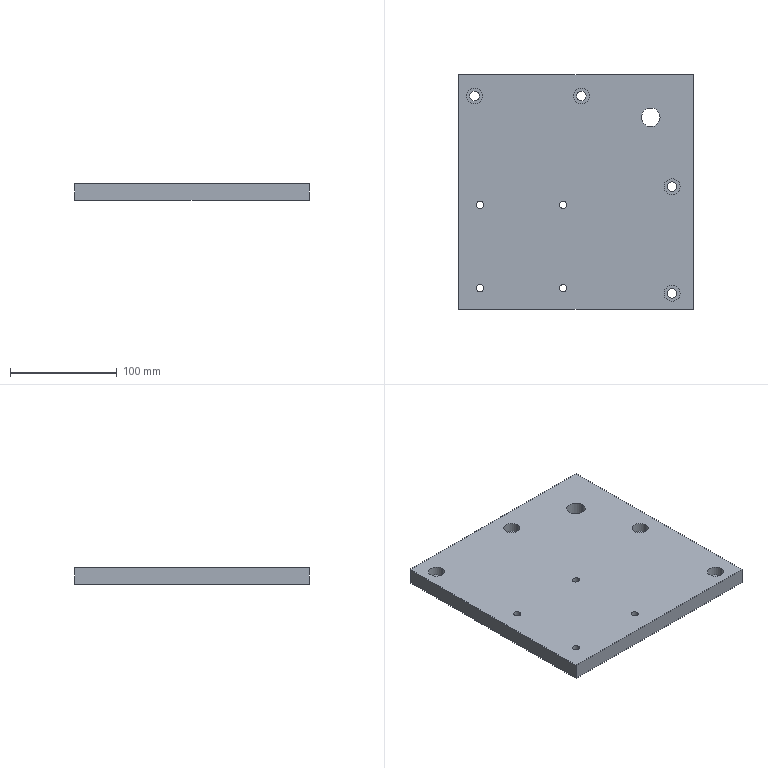Part | SolidWorks | features BaseBody 1 | 1 solid | 36 faces | box 220 x 220 x 15 mm | volume 712325 mm3 | cylinder 26 | plane 10 | commonest cylinder face diameters 6.8 x8 9 x8 15 x8 17.5 x2
STEP:
#1=CARTESIAN_POINT('',(82.5,-95.,6.));
#2=VERTEX_POINT('',#1);
#3=CARTESIAN_POINT('',(97.5,-95.,6.));
#4=VERTEX_POINT('',#3);
#5=CARTESIAN_POINT('',(90.,-95.,6.));
#6=DIRECTION('',(0.,0.,1.));
#7=DIRECTION('',(1.,0.,0.));
#8=AXIS2_PLACEMENT_3D('',#5,#6,#7);
#9=CIRCLE('',#8,7.5);
#10=EDGE_CURVE('',#2,#4,#9,.T.);
#11=ORIENTED_EDGE('',*,*,#10,.F.);
#12=CARTESIAN_POINT('',(82.5,-95.,15.));
#13=VERTEX_POINT('',#12);
#14=CARTESIAN_POINT('',(82.5,-95.,15.));
#15=DIRECTION('',(0.,0.,1.));
#16=VECTOR('',#15,1000.);
#17=LINE('',#14,#16);
#18=EDGE_CURVE('',#2,#13,#17,.T.);
#19=ORIENTED_EDGE('',*,*,#18,.T.);
#20=CARTESIAN_POINT('',(97.5,-95.,15.));
#21=VERTEX_POINT('',#20);
#22=CARTESIAN_POINT('',(90.,-95.,15.));
#23=DIRECTION('',(0.,0.,1.));
#24=DIRECTION('',(1.,0.,0.));
#25=AXIS2_PLACEMENT_3D('',#22,#23,#24);
#26=CIRCLE('',#25,7.5);
#27=EDGE_CURVE('',#13,#21,#26,.T.);
#28=ORIENTED_EDGE('',*,*,#27,.T.);
#29=CARTESIAN_POINT('',(97.5,-95.,15.));
#30=DIRECTION('',(0.,0.,1.));
#31=VECTOR('',#30,1000.);
#32=LINE('',#29,#31);
#33=EDGE_CURVE('',#4,#21,#32,.T.);
#34=ORIENTED_EDGE('',*,*,#33,.F.);
#35=EDGE_LOOP('',(#11,#19,#28,#34));
#36=FACE_OUTER_BOUND('',#35,.T.);
#37=CARTESIAN_POINT('',(90.,-95.,15.));
#38=DIRECTION('',(0.,0.,1.));
#39=DIRECTION('',(1.,0.,0.));
#40=AXIS2_PLACEMENT_3D('',#37,#38,#39);
#41=CYLINDRICAL_SURFACE('',#40,7.5);
#42=ADVANCED_FACE('',(#36),#41,.F.);
#43=CARTESIAN_POINT('',(85.5,-95.,0.));
#44=VERTEX_POINT('',#43);
#45=CARTESIAN_POINT('',(94.5,-95.,0.));
#46=VERTEX_POINT('',#45);
#47=CARTESIAN_POINT('',(90.,-95.,0.));
#48=DIRECTION('',(0.,0.,1.));
#49=DIRECTION('',(1.,0.,0.));
#50=AXIS2_PLACEMENT_3D('',#47,#48,#49);
#51=CIRCLE('',#50,4.5);
#52=EDGE_CURVE('',#44,#46,#51,.T.);
#53=ORIENTED_EDGE('',*,*,#52,.F.);
#54=CARTESIAN_POINT('',(85.5,-95.,6.));
#55=VERTEX_POINT('',#54);
#56=CARTESIAN_POINT('',(85.5,-95.,15.));
#57=DIRECTION('',(0.,0.,1.));
#58=VECTOR('',#57,1000.);
#59=LINE('',#56,#58);
#60=EDGE_CURVE('',#44,#55,#59,.T.);
#61=ORIENTED_EDGE('',*,*,#60,.T.);
#62=CARTESIAN_POINT('',(94.5,-95.,6.));
#63=VERTEX_POINT('',#62);
#64=CARTESIAN_POINT('',(90.,-95.,6.));
#65=DIRECTION('',(0.,0.,1.));
#66=DIRECTION('',(1.,0.,0.));
#67=AXIS2_PLACEMENT_3D('',#64,#65,#66);
#68=CIRCLE('',#67,4.5);
#69=EDGE_CURVE('',#55,#63,#68,.T.);
#70=ORIENTED_EDGE('',*,*,#69,.T.);
#71=CARTESIAN_POINT('',(94.5,-95.,15.));
#72=DIRECTION('',(0.,0.,1.));
#73=VECTOR('',#72,1000.);
#74=LINE('',#71,#73);
#75=EDGE_CURVE('',#46,#63,#74,.T.);
#76=ORIENTED_EDGE('',*,*,#75,.F.);
#77=EDGE_LOOP('',(#53,#61,#70,#76));
#78=FACE_OUTER_BOUND('',#77,.T.);
#79=CARTESIAN_POINT('',(90.,-95.,15.));
#80=DIRECTION('',(0.,0.,1.));
#81=DIRECTION('',(1.,0.,0.));
#82=AXIS2_PLACEMENT_3D('',#79,#80,#81);
#83=CYLINDRICAL_SURFACE('',#82,4.5);
#84=ADVANCED_FACE('',(#78),#83,.F.);
#85=CARTESIAN_POINT('',(82.5,5.,6.));
#86=VERTEX_POINT('',#85);
#87=CARTESIAN_POINT('',(97.5,5.,6.));
#88=VERTEX_POINT('',#87);
#89=CARTESIAN_POINT('',(90.,5.,6.));
#90=DIRECTION('',(0.,0.,1.));
#91=DIRECTION('',(1.,0.,0.));
#92=AXIS2_PLACEMENT_3D('',#89,#90,#91);
#93=CIRCLE('',#92,7.5);
#94=EDGE_CURVE('',#86,#88,#93,.T.);
#95=ORIENTED_EDGE('',*,*,#94,.F.);
#96=CARTESIAN_POINT('',(82.5,5.,15.));
#97=VERTEX_POINT('',#96);
#98=CARTESIAN_POINT('',(82.5,5.,15.));
#99=DIRECTION('',(0.,0.,1.));
#100=VECTOR('',#99,1000.);
#101=LINE('',#98,#100);
#102=EDGE_CURVE('',#86,#97,#101,.T.);
#103=ORIENTED_EDGE('',*,*,#102,.T.);
#104=CARTESIAN_POINT('',(97.5,5.,15.));
#105=VERTEX_POINT('',#104);
#106=CARTESIAN_POINT('',(90.,5.,15.));
#107=DIRECTION('',(0.,0.,1.));
#108=DIRECTION('',(1.,0.,0.));
#109=AXIS2_PLACEMENT_3D('',#106,#107,#108);
#110=CIRCLE('',#109,7.5);
#111=EDGE_CURVE('',#97,#105,#110,.T.);
#112=ORIENTED_EDGE('',*,*,#111,.T.);
#113=CARTESIAN_POINT('',(97.5,5.,15.));
#114=DIRECTION('',(0.,0.,1.));
#115=VECTOR('',#114,1000.);
#116=LINE('',#113,#115);
#117=EDGE_CURVE('',#88,#105,#116,.T.);
#118=ORIENTED_EDGE('',*,*,#117,.F.);
#119=EDGE_LOOP('',(#95,#103,#112,#118));
#120=FACE_OUTER_BOUND('',#119,.T.);
#121=CARTESIAN_POINT('',(90.,5.,15.));
#122=DIRECTION('',(0.,0.,1.));
#123=DIRECTION('',(1.,0.,0.));
#124=AXIS2_PLACEMENT_3D('',#121,#122,#123);
#125=CYLINDRICAL_SURFACE('',#124,7.5);
#126=ADVANCED_FACE('',(#120),#125,.F.);
#127=CARTESIAN_POINT('',(85.5,5.,0.));
#128=VERTEX_POINT('',#127);
#129=CARTESIAN_POINT('',(94.5,5.,0.));
#130=VERTEX_POINT('',#129);
#131=CARTESIAN_POINT('',(90.,5.,0.));
#132=DIRECTION('',(0.,0.,1.));
#133=DIRECTION('',(1.,0.,0.));
#134=AXIS2_PLACEMENT_3D('',#131,#132,#133);
#135=CIRCLE('',#134,4.5);
#136=EDGE_CURVE('',#128,#130,#135,.T.);
#137=ORIENTED_EDGE('',*,*,#136,.F.);
#138=CARTESIAN_POINT('',(85.5,5.,6.));
#139=VERTEX_POINT('',#138);
#140=CARTESIAN_POINT('',(85.5,5.,15.));
#141=DIRECTION('',(0.,0.,1.));
#142=VECTOR('',#141,1000.);
#143=LINE('',#140,#142);
#144=EDGE_CURVE('',#128,#139,#143,.T.);
#145=ORIENTED_EDGE('',*,*,#144,.T.);
#146=CARTESIAN_POINT('',(94.5,5.,6.));
#147=VERTEX_POINT('',#146);
#148=CARTESIAN_POINT('',(90.,5.,6.));
#149=DIRECTION('',(0.,0.,1.));
#150=DIRECTION('',(1.,0.,0.));
#151=AXIS2_PLACEMENT_3D('',#148,#149,#150);
#152=CIRCLE('',#151,4.5);
#153=EDGE_CURVE('',#139,#147,#152,.T.);
#154=ORIENTED_EDGE('',*,*,#153,.T.);
#155=CARTESIAN_POINT('',(94.5,5.,15.));
#156=DIRECTION('',(0.,0.,1.));
#157=VECTOR('',#156,1000.);
#158=LINE('',#155,#157);
#159=EDGE_CURVE('',#130,#147,#158,.T.);
#160=ORIENTED_EDGE('',*,*,#159,.F.);
#161=EDGE_LOOP('',(#137,#145,#154,#160));
#162=FACE_OUTER_BOUND('',#161,.T.);
#163=CARTESIAN_POINT('',(90.,5.,15.));
#164=DIRECTION('',(0.,0.,1.));
#165=DIRECTION('',(1.,0.,0.));
#166=AXIS2_PLACEMENT_3D('',#163,#164,#165);
#167=CYLINDRICAL_SURFACE('',#166,4.5);
#168=ADVANCED_FACE('',(#162),#167,.F.);
#169=CARTESIAN_POINT('',(-102.5,90.,6.));
#170=VERTEX_POINT('',#169);
#171=CARTESIAN_POINT('',(-87.5,90.,6.));
#172=VERTEX_POINT('',#171);
#173=CARTESIAN_POINT('',(-95.,90.,6.));
#174=DIRECTION('',(0.,0.,1.));
#175=DIRECTION('',(1.,0.,0.));
#176=AXIS2_PLACEMENT_3D('',#173,#174,#175);
#177=CIRCLE('',#176,7.5);
#178=EDGE_CURVE('',#170,#172,#177,.T.);
#179=ORIENTED_EDGE('',*,*,#178,.F.);
#180=CARTESIAN_POINT('',(-102.5,90.,15.));
#181=VERTEX_POINT('',#180);
#182=CARTESIAN_POINT('',(-102.5,90.,15.));
#183=DIRECTION('',(0.,0.,1.));
#184=VECTOR('',#183,1000.);
#185=LINE('',#182,#184);
#186=EDGE_CURVE('',#170,#181,#185,.T.);
#187=ORIENTED_EDGE('',*,*,#186,.T.);
#188=CARTESIAN_POINT('',(-87.5,90.,15.));
#189=VERTEX_POINT('',#188);
#190=CARTESIAN_POINT('',(-95.,90.,15.));
#191=DIRECTION('',(0.,0.,1.));
#192=DIRECTION('',(1.,0.,0.));
#193=AXIS2_PLACEMENT_3D('',#190,#191,#192);
#194=CIRCLE('',#193,7.5);
#195=EDGE_CURVE('',#181,#189,#194,.T.);
#196=ORIENTED_EDGE('',*,*,#195,.T.);
#197=CARTESIAN_POINT('',(-87.5,90.,15.));
#198=DIRECTION('',(0.,0.,1.));
#199=VECTOR('',#198,1000.);
#200=LINE('',#197,#199);
#201=EDGE_CURVE('',#172,#189,#200,.T.);
#202=ORIENTED_EDGE('',*,*,#201,.F.);
#203=EDGE_LOOP('',(#179,#187,#196,#202));
#204=FACE_OUTER_BOUND('',#203,.T.);
#205=CARTESIAN_POINT('',(-95.,90.,15.));
#206=DIRECTION('',(0.,0.,1.));
#207=DIRECTION('',(1.,0.,0.));
#208=AXIS2_PLACEMENT_3D('',#205,#206,#207);
#209=CYLINDRICAL_SURFACE('',#208,7.5);
#210=ADVANCED_FACE('',(#204),#209,.F.);
#211=CARTESIAN_POINT('',(-99.5,90.,0.));
#212=VERTEX_POINT('',#211);
#213=CARTESIAN_POINT('',(-90.5,90.,0.));
#214=VERTEX_POINT('',#213);
#215=CARTESIAN_POINT('',(-95.,90.,0.));
#216=DIRECTION('',(0.,0.,1.));
#217=DIRECTION('',(1.,0.,0.));
#218=AXIS2_PLACEMENT_3D('',#215,#216,#217);
#219=CIRCLE('',#218,4.5);
#220=EDGE_CURVE('',#212,#214,#219,.T.);
#221=ORIENTED_EDGE('',*,*,#220,.F.);
#222=CARTESIAN_POINT('',(-99.5,90.,6.));
#223=VERTEX_POINT('',#222);
#224=CARTESIAN_POINT('',(-99.5,90.,15.));
#225=DIRECTION('',(0.,0.,1.));
#226=VECTOR('',#225,1000.);
#227=LINE('',#224,#226);
#228=EDGE_CURVE('',#212,#223,#227,.T.);
#229=ORIENTED_EDGE('',*,*,#228,.T.);
#230=CARTESIAN_POINT('',(-90.5,90.,6.));
#231=VERTEX_POINT('',#230);
#232=CARTESIAN_POINT('',(-95.,90.,6.));
#233=DIRECTION('',(0.,0.,1.));
#234=DIRECTION('',(1.,0.,0.));
#235=AXIS2_PLACEMENT_3D('',#232,#233,#234);
#236=CIRCLE('',#235,4.5);
#237=EDGE_CURVE('',#223,#231,#236,.T.);
#238=ORIENTED_EDGE('',*,*,#237,.T.);
#239=CARTESIAN_POINT('',(-90.5,90.,15.));
#240=DIRECTION('',(0.,0.,1.));
#241=VECTOR('',#240,1000.);
#242=LINE('',#239,#241);
#243=EDGE_CURVE('',#214,#231,#242,.T.);
#244=ORIENTED_EDGE('',*,*,#243,.F.);
#245=EDGE_LOOP('',(#221,#229,#238,#244));
#246=FACE_OUTER_BOUND('',#245,.T.);
#247=CARTESIAN_POINT('',(-95.,90.,15.));
#248=DIRECTION('',(0.,0.,1.));
#249=DIRECTION('',(1.,0.,0.));
#250=AXIS2_PLACEMENT_3D('',#247,#248,#249);
#251=CYLINDRICAL_SURFACE('',#250,4.5);
#252=ADVANCED_FACE('',(#246),#251,.F.);
#253=CARTESIAN_POINT('',(-2.5,90.,6.));
#254=VERTEX_POINT('',#253);
#255=CARTESIAN_POINT('',(12.5,90.,6.));
#256=VERTEX_POINT('',#255);
#257=CARTESIAN_POINT('',(5.,90.,6.));
#258=DIRECTION('',(0.,0.,1.));
#259=DIRECTION('',(1.,0.,0.));
#260=AXIS2_PLACEMENT_3D('',#257,#258,#259);
#261=CIRCLE('',#260,7.5);
#262=EDGE_CURVE('',#254,#256,#261,.T.);
#263=ORIENTED_EDGE('',*,*,#262,.F.);
#264=CARTESIAN_POINT('',(-2.5,90.,15.));
#265=VERTEX_POINT('',#264);
#266=CARTESIAN_POINT('',(-2.5,90.,15.));
#267=DIRECTION('',(0.,0.,1.));
#268=VECTOR('',#267,1000.);
#269=LINE('',#266,#268);
#270=EDGE_CURVE('',#254,#265,#269,.T.);
#271=ORIENTED_EDGE('',*,*,#270,.T.);
#272=CARTESIAN_POINT('',(12.5,90.,15.));
#273=VERTEX_POINT('',#272);
#274=CARTESIAN_POINT('',(5.,90.,15.));
#275=DIRECTION('',(0.,0.,1.));
#276=DIRECTION('',(1.,0.,0.));
#277=AXIS2_PLACEMENT_3D('',#274,#275,#276);
#278=CIRCLE('',#277,7.5);
#279=EDGE_CURVE('',#265,#273,#278,.T.);
#280=ORIENTED_EDGE('',*,*,#279,.T.);
#281=CARTESIAN_POINT('',(12.5,90.,15.));
#282=DIRECTION('',(0.,0.,1.));
#283=VECTOR('',#282,1000.);
#284=LINE('',#281,#283);
#285=EDGE_CURVE('',#256,#273,#284,.T.);
#286=ORIENTED_EDGE('',*,*,#285,.F.);
#287=EDGE_LOOP('',(#263,#271,#280,#286));
#288=FACE_OUTER_BOUND('',#287,.T.);
#289=CARTESIAN_POINT('',(5.,90.,15.));
#290=DIRECTION('',(0.,0.,1.));
#291=DIRECTION('',(1.,0.,0.));
#292=AXIS2_PLACEMENT_3D('',#289,#290,#291);
#293=CYLINDRICAL_SURFACE('',#292,7.5);
#294=ADVANCED_FACE('',(#288),#293,.F.);
#295=CARTESIAN_POINT('',(0.5,90.,0.));
#296=VERTEX_POINT('',#295);
#297=CARTESIAN_POINT('',(9.5,90.,0.));
#298=VERTEX_POINT('',#297);
#299=CARTESIAN_POINT('',(5.,90.,0.));
#300=DIRECTION('',(0.,0.,1.));
#301=DIRECTION('',(1.,0.,0.));
#302=AXIS2_PLACEMENT_3D('',#299,#300,#301);
#303=CIRCLE('',#302,4.5);
#304=EDGE_CURVE('',#296,#298,#303,.T.);
#305=ORIENTED_EDGE('',*,*,#304,.F.);
#306=CARTESIAN_POINT('',(0.5,90.,6.));
#307=VERTEX_POINT('',#306);
#308=CARTESIAN_POINT('',(0.5,90.,15.));
#309=DIRECTION('',(0.,0.,1.));
#310=VECTOR('',#309,1000.);
#311=LINE('',#308,#310);
#312=EDGE_CURVE('',#296,#307,#311,.T.);
#313=ORIENTED_EDGE('',*,*,#312,.T.);
#314=CARTESIAN_POINT('',(9.5,90.,6.));
#315=VERTEX_POINT('',#314);
#316=CARTESIAN_POINT('',(5.,90.,6.));
#317=DIRECTION('',(0.,0.,1.));
#318=DIRECTION('',(1.,0.,0.));
#319=AXIS2_PLACEMENT_3D('',#316,#317,#318);
#320=CIRCLE('',#319,4.5);
#321=EDGE_CURVE('',#307,#315,#320,.T.);
#322=ORIENTED_EDGE('',*,*,#321,.T.);
#323=CARTESIAN_POINT('',(9.5,90.,15.));
#324=DIRECTION('',(0.,0.,1.));
#325=VECTOR('',#324,1000.);
#326=LINE('',#323,#325);
#327=EDGE_CURVE('',#298,#315,#326,.T.);
#328=ORIENTED_EDGE('',*,*,#327,.F.);
#329=EDGE_LOOP('',(#305,#313,#322,#328));
#330=FACE_OUTER_BOUND('',#329,.T.);
#331=CARTESIAN_POINT('',(5.,90.,15.));
#332=DIRECTION('',(0.,0.,1.));
#333=DIRECTION('',(1.,0.,0.));
#334=AXIS2_PLACEMENT_3D('',#331,#332,#333);
#335=CYLINDRICAL_SURFACE('',#334,4.5);
#336=ADVANCED_FACE('',(#330),#335,.F.);
#337=CARTESIAN_POINT('',(61.25,70.,0.));
#338=VERTEX_POINT('',#337);
#339=CARTESIAN_POINT('',(78.75,70.,0.));
#340=VERTEX_POINT('',#339);
#341=CARTESIAN_POINT('',(70.,70.,0.));
#342=DIRECTION('',(0.,0.,1.));
#343=DIRECTION('',(1.,0.,0.));
#344=AXIS2_PLACEMENT_3D('',#341,#342,#343);
#345=CIRCLE('',#344,8.75);
#346=EDGE_CURVE('',#338,#340,#345,.T.);
#347=ORIENTED_EDGE('',*,*,#346,.F.);
#348=CARTESIAN_POINT('',(61.25,70.,15.));
#349=VERTEX_POINT('',#348);
#350=CARTESIAN_POINT('',(61.25,70.,15.));
#351=DIRECTION('',(0.,0.,1.));
#352=VECTOR('',#351,1000.);
#353=LINE('',#350,#352);
#354=EDGE_CURVE('',#338,#349,#353,.T.);
#355=ORIENTED_EDGE('',*,*,#354,.T.);
#356=CARTESIAN_POINT('',(78.75,70.,15.));
#357=VERTEX_POINT('',#356);
#358=CARTESIAN_POINT('',(70.,70.,15.));
#359=DIRECTION('',(0.,0.,1.));
#360=DIRECTION('',(1.,0.,0.));
#361=AXIS2_PLACEMENT_3D('',#358,#359,#360);
#362=CIRCLE('',#361,8.75);
#363=EDGE_CURVE('',#349,#357,#362,.T.);
#364=ORIENTED_EDGE('',*,*,#363,.T.);
#365=CARTESIAN_POINT('',(78.75,70.,15.));
#366=DIRECTION('',(0.,0.,1.));
#367=VECTOR('',#366,1000.);
#368=LINE('',#365,#367);
#369=EDGE_CURVE('',#340,#357,#368,.T.);
#370=ORIENTED_EDGE('',*,*,#369,.F.);
#371=EDGE_LOOP('',(#347,#355,#364,#370));
#372=FACE_OUTER_BOUND('',#371,.T.);
#373=CARTESIAN_POINT('',(70.,70.,15.));
#374=DIRECTION('',(0.,0.,1.));
#375=DIRECTION('',(1.,0.,0.));
#376=AXIS2_PLACEMENT_3D('',#373,#374,#375);
#377=CYLINDRICAL_SURFACE('',#376,8.75);
#378=ADVANCED_FACE('',(#372),#377,.F.);
#379=CARTESIAN_POINT('',(-93.4,-90.,0.));
#380=VERTEX_POINT('',#379);
#381=CARTESIAN_POINT('',(-86.6,-90.,0.));
#382=VERTEX_POINT('',#381);
#383=CARTESIAN_POINT('',(-90.,-90.,0.));
#384=DIRECTION('',(0.,0.,1.));
#385=DIRECTION('',(1.,0.,0.));
#386=AXIS2_PLACEMENT_3D('',#383,#384,#385);
#387=CIRCLE('',#386,3.4);
#388=EDGE_CURVE('',#380,#382,#387,.T.);
#389=ORIENTED_EDGE('',*,*,#388,.F.);
#390=CARTESIAN_POINT('',(-93.4,-90.,15.));
#391=VERTEX_POINT('',#390);
#392=CARTESIAN_POINT('',(-93.4,-90.,15.));
#393=DIRECTION('',(0.,0.,1.));
#394=VECTOR('',#393,1000.);
#395=LINE('',#392,#394);
#396=EDGE_CURVE('',#380,#391,#395,.T.);
#397=ORIENTED_EDGE('',*,*,#396,.T.);
#398=CARTESIAN_POINT('',(-86.6,-90.,15.));
#399=VERTEX_POINT('',#398);
#400=CARTESIAN_POINT('',(-90.,-90.,15.));
#401=DIRECTION('',(0.,0.,1.));
#402=DIRECTION('',(1.,0.,0.));
#403=AXIS2_PLACEMENT_3D('',#400,#401,#402);
#404=CIRCLE('',#403,3.4);
#405=EDGE_CURVE('',#391,#399,#404,.T.);
#406=ORIENTED_EDGE('',*,*,#405,.T.);
#407=CARTESIAN_POINT('',(-86.6,-90.,15.));
#408=DIRECTION('',(0.,0.,1.));
#409=VECTOR('',#408,1000.);
#410=LINE('',#407,#409);
#411=EDGE_CURVE('',#382,#399,#410,.T.);
#412=ORIENTED_EDGE('',*,*,#411,.F.);
#413=EDGE_LOOP('',(#389,#397,#406,#412));
#414=FACE_OUTER_BOUND('',#413,.T.);
#415=CARTESIAN_POINT('',(-90.,-90.,15.));
#416=DIRECTION('',(0.,0.,1.));
#417=DIRECTION('',(1.,0.,0.));
#418=AXIS2_PLACEMENT_3D('',#415,#416,#417);
#419=CYLINDRICAL_SURFACE('',#418,3.4);
#420=ADVANCED_FACE('',(#414),#419,.F.);
#421=CARTESIAN_POINT('',(-93.4,-12.,0.));
#422=VERTEX_POINT('',#421);
#423=CARTESIAN_POINT('',(-86.6,-12.,0.));
#424=VERTEX_POINT('',#423);
#425=CARTESIAN_POINT('',(-90.,-12.,0.));
#426=DIRECTION('',(0.,0.,1.));
#427=DIRECTION('',(1.,0.,0.));
#428=AXIS2_PLACEMENT_3D('',#425,#426,#427);
#429=CIRCLE('',#428,3.4);
#430=EDGE_CURVE('',#422,#424,#429,.T.);
#431=ORIENTED_EDGE('',*,*,#430,.F.);
#432=CARTESIAN_POINT('',(-93.4,-12.,15.));
#433=VERTEX_POINT('',#432);
#434=CARTESIAN_POINT('',(-93.4,-12.,15.));
#435=DIRECTION('',(0.,0.,1.));
#436=VECTOR('',#435,1000.);
#437=LINE('',#434,#436);
#438=EDGE_CURVE('',#422,#433,#437,.T.);
#439=ORIENTED_EDGE('',*,*,#438,.T.);
#440=CARTESIAN_POINT('',(-86.6,-12.,15.));
#441=VERTEX_POINT('',#440);
#442=CARTESIAN_POINT('',(-90.,-12.,15.));
#443=DIRECTION('',(0.,0.,1.));
#444=DIRECTION('',(1.,0.,0.));
#445=AXIS2_PLACEMENT_3D('',#442,#443,#444);
#446=CIRCLE('',#445,3.4);
#447=EDGE_CURVE('',#433,#441,#446,.T.);
#448=ORIENTED_EDGE('',*,*,#447,.T.);
#449=CARTESIAN_POINT('',(-86.6,-12.,15.));
#450=DIRECTION('',(0.,0.,1.));
#451=VECTOR('',#450,1000.);
#452=LINE('',#449,#451);
#453=EDGE_CURVE('',#424,#441,#452,.T.);
#454=ORIENTED_EDGE('',*,*,#453,.F.);
#455=EDGE_LOOP('',(#431,#439,#448,#454));
#456=FACE_OUTER_BOUND('',#455,.T.);
#457=CARTESIAN_POINT('',(-90.,-12.,15.));
#458=DIRECTION('',(0.,0.,1.));
#459=DIRECTION('',(1.,0.,0.));
#460=AXIS2_PLACEMENT_3D('',#457,#458,#459);
#461=CYLINDRICAL_SURFACE('',#460,3.4);
#462=ADVANCED_FACE('',(#456),#461,.F.);
#463=CARTESIAN_POINT('',(-15.4,-12.,0.));
#464=VERTEX_POINT('',#463);
#465=CARTESIAN_POINT('',(-8.6,-12.,0.));
#466=VERTEX_POINT('',#465);
#467=CARTESIAN_POINT('',(-12.,-12.,0.));
#468=DIRECTION('',(0.,0.,1.));
#469=DIRECTION('',(1.,0.,0.));
#470=AXIS2_PLACEMENT_3D('',#467,#468,#469);
#471=CIRCLE('',#470,3.4);
#472=EDGE_CURVE('',#464,#466,#471,.T.);
#473=ORIENTED_EDGE('',*,*,#472,.F.);
#474=CARTESIAN_POINT('',(-15.4,-12.,15.));
#475=VERTEX_POINT('',#474);
#476=CARTESIAN_POINT('',(-15.4,-12.,15.));
#477=DIRECTION('',(0.,0.,1.));
#478=VECTOR('',#477,1000.);
#479=LINE('',#476,#478);
#480=EDGE_CURVE('',#464,#475,#479,.T.);
#481=ORIENTED_EDGE('',*,*,#480,.T.);
#482=CARTESIAN_POINT('',(-8.6,-12.,15.));
#483=VERTEX_POINT('',#482);
#484=CARTESIAN_POINT('',(-12.,-12.,15.));
#485=DIRECTION('',(0.,0.,1.));
#486=DIRECTION('',(1.,0.,0.));
#487=AXIS2_PLACEMENT_3D('',#484,#485,#486);
#488=CIRCLE('',#487,3.4);
#489=EDGE_CURVE('',#475,#483,#488,.T.);
#490=ORIENTED_EDGE('',*,*,#489,.T.);
#491=CARTESIAN_POINT('',(-8.6,-12.,15.));
#492=DIRECTION('',(0.,0.,1.));
#493=VECTOR('',#492,1000.);
#494=LINE('',#491,#493);
#495=EDGE_CURVE('',#466,#483,#494,.T.);
#496=ORIENTED_EDGE('',*,*,#495,.F.);
#497=EDGE_LOOP('',(#473,#481,#490,#496));
#498=FACE_OUTER_BOUND('',#497,.T.);
#499=CARTESIAN_POINT('',(-12.,-12.,15.));
#500=DIRECTION('',(0.,0.,1.));
#501=DIRECTION('',(1.,0.,0.));
#502=AXIS2_PLACEMENT_3D('',#499,#500,#501);
#503=CYLINDRICAL_SURFACE('',#502,3.4);
#504=ADVANCED_FACE('',(#498),#503,.F.);
#505=CARTESIAN_POINT('',(-15.4,-90.,0.));
#506=VERTEX_POINT('',#505);
#507=CARTESIAN_POINT('',(-8.6,-90.,0.));
#508=VERTEX_POINT('',#507);
#509=CARTESIAN_POINT('',(-12.,-90.,0.));
#510=DIRECTION('',(0.,0.,1.));
#511=DIRECTION('',(1.,0.,0.));
#512=AXIS2_PLACEMENT_3D('',#509,#510,#511);
#513=CIRCLE('',#512,3.4);
#514=EDGE_CURVE('',#506,#508,#513,.T.);
#515=ORIENTED_EDGE('',*,*,#514,.F.);
#516=CARTESIAN_POINT('',(-15.4,-90.,15.));
#517=VERTEX_POINT('',#516);
#518=CARTESIAN_POINT('',(-15.4,-90.,15.));
#519=DIRECTION('',(0.,0.,1.));
#520=VECTOR('',#519,1000.);
#521=LINE('',#518,#520);
#522=EDGE_CURVE('',#506,#517,#521,.T.);
#523=ORIENTED_EDGE('',*,*,#522,.T.);
#524=CARTESIAN_POINT('',(-8.6,-90.,15.));
#525=VERTEX_POINT('',#524);
#526=CARTESIAN_POINT('',(-12.,-90.,15.));
#527=DIRECTION('',(0.,0.,1.));
#528=DIRECTION('',(1.,0.,0.));
#529=AXIS2_PLACEMENT_3D('',#526,#527,#528);
#530=CIRCLE('',#529,3.4);
#531=EDGE_CURVE('',#517,#525,#530,.T.);
#532=ORIENTED_EDGE('',*,*,#531,.T.);
#533=CARTESIAN_POINT('',(-8.6,-90.,15.));
#534=DIRECTION('',(0.,0.,1.));
#535=VECTOR('',#534,1000.);
#536=LINE('',#533,#535);
#537=EDGE_CURVE('',#508,#525,#536,.T.);
#538=ORIENTED_EDGE('',*,*,#537,.F.);
#539=EDGE_LOOP('',(#515,#523,#532,#538));
#540=FACE_OUTER_BOUND('',#539,.T.);
#541=CARTESIAN_POINT('',(-12.,-90.,15.));
#542=DIRECTION('',(0.,0.,1.));
#543=DIRECTION('',(1.,0.,0.));
#544=AXIS2_PLACEMENT_3D('',#541,#542,#543);
#545=CYLINDRICAL_SURFACE('',#544,3.4);
#546=ADVANCED_FACE('',(#540),#545,.F.);
#547=CARTESIAN_POINT('',(90.,-95.,6.));
#548=DIRECTION('',(0.,0.,1.));
#549=DIRECTION('',(1.,0.,0.));
#550=AXIS2_PLACEMENT_3D('',#547,#548,#549);
#551=CIRCLE('',#550,4.5);
#552=EDGE_CURVE('',#63,#55,#551,.T.);
#553=ORIENTED_EDGE('',*,*,#552,.F.);
#554=ORIENTED_EDGE('',*,*,#69,.F.);
#555=EDGE_LOOP('',(#553,#554));
#556=FACE_BOUND('',#555,.T.);
#557=CARTESIAN_POINT('',(90.,-95.,6.));
#558=DIRECTION('',(0.,0.,1.));
#559=DIRECTION('',(1.,0.,0.));
#560=AXIS2_PLACEMENT_3D('',#557,#558,#559);
#561=CIRCLE('',#560,7.5);
#562=EDGE_CURVE('',#4,#2,#561,.T.);
#563=ORIENTED_EDGE('',*,*,#562,.T.);
#564=ORIENTED_EDGE('',*,*,#10,.T.);
#565=EDGE_LOOP('',(#563,#564));
#566=FACE_OUTER_BOUND('',#565,.T.);
#567=CARTESIAN_POINT('',(94.5,-95.,6.));
#568=DIRECTION('',(0.,0.,-1.));
#569=DIRECTION('',(0.,-1.,0.));
#570=AXIS2_PLACEMENT_3D('',#567,#568,#569);
#571=PLANE('',#570);
#572=ADVANCED_FACE('',(#556,#566),#571,.F.);
#573=CARTESIAN_POINT('',(90.,5.,6.));
#574=DIRECTION('',(0.,0.,1.));
#575=DIRECTION('',(1.,0.,0.));
#576=AXIS2_PLACEMENT_3D('',#573,#574,#575);
#577=CIRCLE('',#576,4.5);
#578=EDGE_CURVE('',#147,#139,#577,.T.);
#579=ORIENTED_EDGE('',*,*,#578,.F.);
#580=ORIENTED_EDGE('',*,*,#153,.F.);
#581=EDGE_LOOP('',(#579,#580));
#582=FACE_BOUND('',#581,.T.);
#583=CARTESIAN_POINT('',(90.,5.,6.));
#584=DIRECTION('',(0.,0.,1.));
#585=DIRECTION('',(1.,0.,0.));
#586=AXIS2_PLACEMENT_3D('',#583,#584,#585);
#587=CIRCLE('',#586,7.5);
#588=EDGE_CURVE('',#88,#86,#587,.T.);
#589=ORIENTED_EDGE('',*,*,#588,.T.);
#590=ORIENTED_EDGE('',*,*,#94,.T.);
#591=EDGE_LOOP('',(#589,#590));
#592=FACE_OUTER_BOUND('',#591,.T.);
#593=CARTESIAN_POINT('',(94.5,5.,6.));
#594=DIRECTION('',(0.,0.,-1.));
#595=DIRECTION('',(0.,-1.,0.));
#596=AXIS2_PLACEMENT_3D('',#593,#594,#595);
#597=PLANE('',#596);
#598=ADVANCED_FACE('',(#582,#592),#597,.F.);
#599=CARTESIAN_POINT('',(-95.,90.,6.));
#600=DIRECTION('',(0.,0.,1.));
#601=DIRECTION('',(1.,0.,0.));
#602=AXIS2_PLACEMENT_3D('',#599,#600,#601);
#603=CIRCLE('',#602,4.5);
#604=EDGE_CURVE('',#231,#223,#603,.T.);
#605=ORIENTED_EDGE('',*,*,#604,.F.);
#606=ORIENTED_EDGE('',*,*,#237,.F.);
#607=EDGE_LOOP('',(#605,#606));
#608=FACE_BOUND('',#607,.T.);
#609=CARTESIAN_POINT('',(-95.,90.,6.));
#610=DIRECTION('',(0.,0.,1.));
#611=DIRECTION('',(1.,0.,0.));
#612=AXIS2_PLACEMENT_3D('',#609,#610,#611);
#613=CIRCLE('',#612,7.5);
#614=EDGE_CURVE('',#172,#170,#613,.T.);
#615=ORIENTED_EDGE('',*,*,#614,.T.);
#616=ORIENTED_EDGE('',*,*,#178,.T.);
#617=EDGE_LOOP('',(#615,#616));
#618=FACE_OUTER_BOUND('',#617,.T.);
#619=CARTESIAN_POINT('',(-90.5,90.,6.));
#620=DIRECTION('',(0.,0.,-1.));
#621=DIRECTION('',(0.,-1.,0.));
#622=AXIS2_PLACEMENT_3D('',#619,#620,#621);
#623=PLANE('',#622);
#624=ADVANCED_FACE('',(#608,#618),#623,.F.);
#625=CARTESIAN_POINT('',(5.,90.,6.));
#626=DIRECTION('',(0.,0.,1.));
#627=DIRECTION('',(1.,0.,0.));
#628=AXIS2_PLACEMENT_3D('',#625,#626,#627);
#629=CIRCLE('',#628,4.5);
#630=EDGE_CURVE('',#315,#307,#629,.T.);
#631=ORIENTED_EDGE('',*,*,#630,.F.);
#632=ORIENTED_EDGE('',*,*,#321,.F.);
#633=EDGE_LOOP('',(#631,#632));
#634=FACE_BOUND('',#633,.T.);
#635=CARTESIAN_POINT('',(5.,90.,6.));
#636=DIRECTION('',(0.,0.,1.));
#637=DIRECTION('',(1.,0.,0.));
#638=AXIS2_PLACEMENT_3D('',#635,#636,#637);
#639=CIRCLE('',#638,7.5);
#640=EDGE_CURVE('',#256,#254,#639,.T.);
#641=ORIENTED_EDGE('',*,*,#640,.T.);
#642=ORIENTED_EDGE('',*,*,#262,.T.);
#643=EDGE_LOOP('',(#641,#642));
#644=FACE_OUTER_BOUND('',#643,.T.);
#645=CARTESIAN_POINT('',(9.5,90.,6.));
#646=DIRECTION('',(0.,0.,-1.));
#647=DIRECTION('',(0.,-1.,0.));
#648=AXIS2_PLACEMENT_3D('',#645,#646,#647);
#649=PLANE('',#648);
#650=ADVANCED_FACE('',(#634,#644),#649,.F.);
#651=CARTESIAN_POINT('',(-12.,-90.,0.));
#652=DIRECTION('',(0.,0.,1.));
#653=DIRECTION('',(1.,0.,0.));
#654=AXIS2_PLACEMENT_3D('',#651,#652,#653);
#655=CIRCLE('',#654,3.4);
#656=EDGE_CURVE('',#508,#506,#655,.T.);
#657=ORIENTED_EDGE('',*,*,#656,.T.);
#658=ORIENTED_EDGE('',*,*,#514,.T.);
#659=EDGE_LOOP('',(#657,#658));
#660=FACE_BOUND('',#659,.T.);
#661=CARTESIAN_POINT('',(-12.,-12.,0.));
#662=DIRECTION('',(0.,0.,1.));
#663=DIRECTION('',(1.,0.,0.));
#664=AXIS2_PLACEMENT_3D('',#661,#662,#663);
#665=CIRCLE('',#664,3.4);
#666=EDGE_CURVE('',#466,#464,#665,.T.);
#667=ORIENTED_EDGE('',*,*,#666,.T.);
#668=ORIENTED_EDGE('',*,*,#472,.T.);
#669=EDGE_LOOP('',(#667,#668));
#670=FACE_BOUND('',#669,.T.);
#671=CARTESIAN_POINT('',(-90.,-12.,0.));
#672=DIRECTION('',(0.,0.,1.));
#673=DIRECTION('',(1.,0.,0.));
#674=AXIS2_PLACEMENT_3D('',#671,#672,#673);
#675=CIRCLE('',#674,3.4);
#676=EDGE_CURVE('',#424,#422,#675,.T.);
#677=ORIENTED_EDGE('',*,*,#676,.T.);
#678=ORIENTED_EDGE('',*,*,#430,.T.);
#679=EDGE_LOOP('',(#677,#678));
#680=FACE_BOUND('',#679,.T.);
#681=CARTESIAN_POINT('',(-90.,-90.,0.));
#682=DIRECTION('',(0.,0.,1.));
#683=DIRECTION('',(1.,0.,0.));
#684=AXIS2_PLACEMENT_3D('',#681,#682,#683);
#685=CIRCLE('',#684,3.4);
#686=EDGE_CURVE('',#382,#380,#685,.T.);
#687=ORIENTED_EDGE('',*,*,#686,.T.);
#688=ORIENTED_EDGE('',*,*,#388,.T.);
#689=EDGE_LOOP('',(#687,#688));
#690=FACE_BOUND('',#689,.T.);
#691=CARTESIAN_POINT('',(70.,70.,0.));
#692=DIRECTION('',(0.,0.,1.));
#693=DIRECTION('',(1.,0.,0.));
#694=AXIS2_PLACEMENT_3D('',#691,#692,#693);
#695=CIRCLE('',#694,8.75);
#696=EDGE_CURVE('',#340,#338,#695,.T.);
#697=ORIENTED_EDGE('',*,*,#696,.T.);
#698=ORIENTED_EDGE('',*,*,#346,.T.);
#699=EDGE_LOOP('',(#697,#698));
#700=FACE_BOUND('',#699,.T.);
#701=CARTESIAN_POINT('',(5.,90.,0.));
#702=DIRECTION('',(0.,0.,1.));
#703=DIRECTION('',(1.,0.,0.));
#704=AXIS2_PLACEMENT_3D('',#701,#702,#703);
#705=CIRCLE('',#704,4.5);
#706=EDGE_CURVE('',#298,#296,#705,.T.);
#707=ORIENTED_EDGE('',*,*,#706,.T.);
#708=ORIENTED_EDGE('',*,*,#304,.T.);
#709=EDGE_LOOP('',(#707,#708));
#710=FACE_BOUND('',#709,.T.);
#711=CARTESIAN_POINT('',(-95.,90.,0.));
#712=DIRECTION('',(0.,0.,1.));
#713=DIRECTION('',(1.,0.,0.));
#714=AXIS2_PLACEMENT_3D('',#711,#712,#713);
#715=CIRCLE('',#714,4.5);
#716=EDGE_CURVE('',#214,#212,#715,.T.);
#717=ORIENTED_EDGE('',*,*,#716,.T.);
#718=ORIENTED_EDGE('',*,*,#220,.T.);
#719=EDGE_LOOP('',(#717,#718));
#720=FACE_BOUND('',#719,.T.);
#721=CARTESIAN_POINT('',(90.,5.,0.));
#722=DIRECTION('',(0.,0.,1.));
#723=DIRECTION('',(1.,0.,0.));
#724=AXIS2_PLACEMENT_3D('',#721,#722,#723);
#725=CIRCLE('',#724,4.5);
#726=EDGE_CURVE('',#130,#128,#725,.T.);
#727=ORIENTED_EDGE('',*,*,#726,.T.);
#728=ORIENTED_EDGE('',*,*,#136,.T.);
#729=EDGE_LOOP('',(#727,#728));
#730=FACE_BOUND('',#729,.T.);
#731=CARTESIAN_POINT('',(90.,-95.,0.));
#732=DIRECTION('',(0.,0.,1.));
#733=DIRECTION('',(1.,0.,0.));
#734=AXIS2_PLACEMENT_3D('',#731,#732,#733);
#735=CIRCLE('',#734,4.5);
#736=EDGE_CURVE('',#46,#44,#735,.T.);
#737=ORIENTED_EDGE('',*,*,#736,.T.);
#738=ORIENTED_EDGE('',*,*,#52,.T.);
#739=EDGE_LOOP('',(#737,#738));
#740=FACE_BOUND('',#739,.T.);
#741=CARTESIAN_POINT('',(110.,-110.,0.));
#742=VERTEX_POINT('',#741);
#743=CARTESIAN_POINT('',(110.,110.,0.));
#744=VERTEX_POINT('',#743);
#745=CARTESIAN_POINT('',(110.,110.,0.));
#746=DIRECTION('',(0.,1.,0.));
#747=VECTOR('',#746,1000.);
#748=LINE('',#745,#747);
#749=EDGE_CURVE('',#742,#744,#748,.T.);
#750=ORIENTED_EDGE('',*,*,#749,.F.);
#751=CARTESIAN_POINT('',(-110.,-110.,0.));
#752=VERTEX_POINT('',#751);
#753=CARTESIAN_POINT('',(-110.,-110.,0.));
#754=DIRECTION('',(1.,0.,0.));
#755=VECTOR('',#754,1000.);
#756=LINE('',#753,#755);
#757=EDGE_CURVE('',#752,#742,#756,.T.);
#758=ORIENTED_EDGE('',*,*,#757,.F.);
#759=CARTESIAN_POINT('',(-110.,110.,0.));
#760=VERTEX_POINT('',#759);
#761=CARTESIAN_POINT('',(-110.,110.,0.));
#762=DIRECTION('',(0.,-1.,0.));
#763=VECTOR('',#762,1000.);
#764=LINE('',#761,#763);
#765=EDGE_CURVE('',#760,#752,#764,.T.);
#766=ORIENTED_EDGE('',*,*,#765,.F.);
#767=CARTESIAN_POINT('',(-110.,110.,0.));
#768=DIRECTION('',(-1.,0.,0.));
#769=VECTOR('',#768,1000.);
#770=LINE('',#767,#769);
#771=EDGE_CURVE('',#744,#760,#770,.T.);
#772=ORIENTED_EDGE('',*,*,#771,.F.);
#773=EDGE_LOOP('',(#750,#758,#766,#772));
#774=FACE_OUTER_BOUND('',#773,.T.);
#775=CARTESIAN_POINT('',(0.,0.,0.));
#776=DIRECTION('',(0.,0.,1.));
#777=DIRECTION('',(1.,0.,0.));
#778=AXIS2_PLACEMENT_3D('',#775,#776,#777);
#779=PLANE('',#778);
#780=ADVANCED_FACE('',(#660,#670,#680,#690,#700,#710,#720,#730,#740,#774),#779,.F.);
#781=CARTESIAN_POINT('',(-12.,-90.,15.));
#782=DIRECTION('',(0.,0.,1.));
#783=DIRECTION('',(1.,0.,0.));
#784=AXIS2_PLACEMENT_3D('',#781,#782,#783);
#785=CIRCLE('',#784,3.4);
#786=EDGE_CURVE('',#525,#517,#785,.T.);
#787=ORIENTED_EDGE('',*,*,#786,.F.);
#788=ORIENTED_EDGE('',*,*,#531,.F.);
#789=EDGE_LOOP('',(#787,#788));
#790=FACE_BOUND('',#789,.T.);
#791=CARTESIAN_POINT('',(-12.,-12.,15.));
#792=DIRECTION('',(0.,0.,1.));
#793=DIRECTION('',(1.,0.,0.));
#794=AXIS2_PLACEMENT_3D('',#791,#792,#793);
#795=CIRCLE('',#794,3.4);
#796=EDGE_CURVE('',#483,#475,#795,.T.);
#797=ORIENTED_EDGE('',*,*,#796,.F.);
#798=ORIENTED_EDGE('',*,*,#489,.F.);
#799=EDGE_LOOP('',(#797,#798));
#800=FACE_BOUND('',#799,.T.);
#801=CARTESIAN_POINT('',(-90.,-12.,15.));
#802=DIRECTION('',(0.,0.,1.));
#803=DIRECTION('',(1.,0.,0.));
#804=AXIS2_PLACEMENT_3D('',#801,#802,#803);
#805=CIRCLE('',#804,3.4);
#806=EDGE_CURVE('',#441,#433,#805,.T.);
#807=ORIENTED_EDGE('',*,*,#806,.F.);
#808=ORIENTED_EDGE('',*,*,#447,.F.);
#809=EDGE_LOOP('',(#807,#808));
#810=FACE_BOUND('',#809,.T.);
#811=CARTESIAN_POINT('',(-90.,-90.,15.));
#812=DIRECTION('',(0.,0.,1.));
#813=DIRECTION('',(1.,0.,0.));
#814=AXIS2_PLACEMENT_3D('',#811,#812,#813);
#815=CIRCLE('',#814,3.4);
#816=EDGE_CURVE('',#399,#391,#815,.T.);
#817=ORIENTED_EDGE('',*,*,#816,.F.);
#818=ORIENTED_EDGE('',*,*,#405,.F.);
#819=EDGE_LOOP('',(#817,#818));
#820=FACE_BOUND('',#819,.T.);
#821=CARTESIAN_POINT('',(70.,70.,15.));
#822=DIRECTION('',(0.,0.,1.));
#823=DIRECTION('',(1.,0.,0.));
#824=AXIS2_PLACEMENT_3D('',#821,#822,#823);
#825=CIRCLE('',#824,8.75);
#826=EDGE_CURVE('',#357,#349,#825,.T.);
#827=ORIENTED_EDGE('',*,*,#826,.F.);
#828=ORIENTED_EDGE('',*,*,#363,.F.);
#829=EDGE_LOOP('',(#827,#828));
#830=FACE_BOUND('',#829,.T.);
#831=CARTESIAN_POINT('',(5.,90.,15.));
#832=DIRECTION('',(0.,0.,1.));
#833=DIRECTION('',(1.,0.,0.));
#834=AXIS2_PLACEMENT_3D('',#831,#832,#833);
#835=CIRCLE('',#834,7.5);
#836=EDGE_CURVE('',#273,#265,#835,.T.);
#837=ORIENTED_EDGE('',*,*,#836,.F.);
#838=ORIENTED_EDGE('',*,*,#279,.F.);
#839=EDGE_LOOP('',(#837,#838));
#840=FACE_BOUND('',#839,.T.);
#841=CARTESIAN_POINT('',(-95.,90.,15.));
#842=DIRECTION('',(0.,0.,1.));
#843=DIRECTION('',(1.,0.,0.));
#844=AXIS2_PLACEMENT_3D('',#841,#842,#843);
#845=CIRCLE('',#844,7.5);
#846=EDGE_CURVE('',#189,#181,#845,.T.);
#847=ORIENTED_EDGE('',*,*,#846,.F.);
#848=ORIENTED_EDGE('',*,*,#195,.F.);
#849=EDGE_LOOP('',(#847,#848));
#850=FACE_BOUND('',#849,.T.);
#851=CARTESIAN_POINT('',(90.,5.,15.));
#852=DIRECTION('',(0.,0.,1.));
#853=DIRECTION('',(1.,0.,0.));
#854=AXIS2_PLACEMENT_3D('',#851,#852,#853);
#855=CIRCLE('',#854,7.5);
#856=EDGE_CURVE('',#105,#97,#855,.T.);
#857=ORIENTED_EDGE('',*,*,#856,.F.);
#858=ORIENTED_EDGE('',*,*,#111,.F.);
#859=EDGE_LOOP('',(#857,#858));
#860=FACE_BOUND('',#859,.T.);
#861=CARTESIAN_POINT('',(90.,-95.,15.));
#862=DIRECTION('',(0.,0.,1.));
#863=DIRECTION('',(1.,0.,0.));
#864=AXIS2_PLACEMENT_3D('',#861,#862,#863);
#865=CIRCLE('',#864,7.5);
#866=EDGE_CURVE('',#21,#13,#865,.T.);
#867=ORIENTED_EDGE('',*,*,#866,.F.);
#868=ORIENTED_EDGE('',*,*,#27,.F.);
#869=EDGE_LOOP('',(#867,#868));
#870=FACE_BOUND('',#869,.T.);
#871=CARTESIAN_POINT('',(110.,-110.,15.));
#872=VERTEX_POINT('',#871);
#873=CARTESIAN_POINT('',(110.,110.,15.));
#874=VERTEX_POINT('',#873);
#875=CARTESIAN_POINT('',(110.,110.,15.));
#876=DIRECTION('',(0.,1.,0.));
#877=VECTOR('',#876,1000.);
#878=LINE('',#875,#877);
#879=EDGE_CURVE('',#872,#874,#878,.T.);
#880=ORIENTED_EDGE('',*,*,#879,.T.);
#881=CARTESIAN_POINT('',(-110.,110.,15.));
#882=VERTEX_POINT('',#881);
#883=CARTESIAN_POINT('',(-110.,110.,15.));
#884=DIRECTION('',(-1.,0.,0.));
#885=VECTOR('',#884,1000.);
#886=LINE('',#883,#885);
#887=EDGE_CURVE('',#874,#882,#886,.T.);
#888=ORIENTED_EDGE('',*,*,#887,.T.);
#889=CARTESIAN_POINT('',(-110.,-110.,15.));
#890=VERTEX_POINT('',#889);
#891=CARTESIAN_POINT('',(-110.,110.,15.));
#892=DIRECTION('',(0.,-1.,0.));
#893=VECTOR('',#892,1000.);
#894=LINE('',#891,#893);
#895=EDGE_CURVE('',#882,#890,#894,.T.);
#896=ORIENTED_EDGE('',*,*,#895,.T.);
#897=CARTESIAN_POINT('',(-110.,-110.,15.));
#898=DIRECTION('',(1.,0.,0.));
#899=VECTOR('',#898,1000.);
#900=LINE('',#897,#899);
#901=EDGE_CURVE('',#890,#872,#900,.T.);
#902=ORIENTED_EDGE('',*,*,#901,.T.);
#903=EDGE_LOOP('',(#880,#888,#896,#902));
#904=FACE_OUTER_BOUND('',#903,.T.);
#905=CARTESIAN_POINT('',(0.,0.,15.));
#906=DIRECTION('',(0.,0.,1.));
#907=DIRECTION('',(1.,0.,0.));
#908=AXIS2_PLACEMENT_3D('',#905,#906,#907);
#909=PLANE('',#908);
#910=ADVANCED_FACE('',(#790,#800,#810,#820,#830,#840,#850,#860,#870,#904),#909,.T.);
#911=ORIENTED_EDGE('',*,*,#757,.T.);
#912=CARTESIAN_POINT('',(110.,-110.,15.));
#913=DIRECTION('',(0.,0.,-1.));
#914=VECTOR('',#913,1000.);
#915=LINE('',#912,#914);
#916=EDGE_CURVE('',#872,#742,#915,.T.);
#917=ORIENTED_EDGE('',*,*,#916,.F.);
#918=ORIENTED_EDGE('',*,*,#901,.F.);
#919=CARTESIAN_POINT('',(-110.,-110.,15.));
#920=DIRECTION('',(0.,0.,-1.));
#921=VECTOR('',#920,1000.);
#922=LINE('',#919,#921);
#923=EDGE_CURVE('',#890,#752,#922,.T.);
#924=ORIENTED_EDGE('',*,*,#923,.T.);
#925=EDGE_LOOP('',(#911,#917,#918,#924));
#926=FACE_OUTER_BOUND('',#925,.T.);
#927=CARTESIAN_POINT('',(-110.,-110.,15.));
#928=DIRECTION('',(0.,1.,0.));
#929=DIRECTION('',(1.,0.,0.));
#930=AXIS2_PLACEMENT_3D('',#927,#928,#929);
#931=PLANE('',#930);
#932=ADVANCED_FACE('',(#926),#931,.F.);
#933=ORIENTED_EDGE('',*,*,#765,.T.);
#934=ORIENTED_EDGE('',*,*,#923,.F.);
#935=ORIENTED_EDGE('',*,*,#895,.F.);
#936=CARTESIAN_POINT('',(-110.,110.,15.));
#937=DIRECTION('',(0.,0.,-1.));
#938=VECTOR('',#937,1000.);
#939=LINE('',#936,#938);
#940=EDGE_CURVE('',#882,#760,#939,.T.);
#941=ORIENTED_EDGE('',*,*,#940,.T.);
#942=EDGE_LOOP('',(#933,#934,#935,#941));
#943=FACE_OUTER_BOUND('',#942,.T.);
#944=CARTESIAN_POINT('',(-110.,110.,15.));
#945=DIRECTION('',(1.,0.,0.));
#946=DIRECTION('',(0.,1.,0.));
#947=AXIS2_PLACEMENT_3D('',#944,#945,#946);
#948=PLANE('',#947);
#949=ADVANCED_FACE('',(#943),#948,.F.);
#950=ORIENTED_EDGE('',*,*,#771,.T.);
#951=ORIENTED_EDGE('',*,*,#940,.F.);
#952=ORIENTED_EDGE('',*,*,#887,.F.);
#953=CARTESIAN_POINT('',(110.,110.,15.));
#954=DIRECTION('',(0.,0.,-1.));
#955=VECTOR('',#954,1000.);
#956=LINE('',#953,#955);
#957=EDGE_CURVE('',#874,#744,#956,.T.);
#958=ORIENTED_EDGE('',*,*,#957,.T.);
#959=EDGE_LOOP('',(#950,#951,#952,#958));
#960=FACE_OUTER_BOUND('',#959,.T.);
#961=CARTESIAN_POINT('',(-110.,110.,15.));
#962=DIRECTION('',(0.,-1.,0.));
#963=DIRECTION('',(0.,0.,-1.));
#964=AXIS2_PLACEMENT_3D('',#961,#962,#963);
#965=PLANE('',#964);
#966=ADVANCED_FACE('',(#960),#965,.F.);
#967=ORIENTED_EDGE('',*,*,#749,.T.);
#968=ORIENTED_EDGE('',*,*,#957,.F.);
#969=ORIENTED_EDGE('',*,*,#879,.F.);
#970=ORIENTED_EDGE('',*,*,#916,.T.);
#971=EDGE_LOOP('',(#967,#968,#969,#970));
#972=FACE_OUTER_BOUND('',#971,.T.);
#973=CARTESIAN_POINT('',(110.,110.,15.));
#974=DIRECTION('',(-1.,0.,0.));
#975=DIRECTION('',(0.,1.,0.));
#976=AXIS2_PLACEMENT_3D('',#973,#974,#975);
#977=PLANE('',#976);
#978=ADVANCED_FACE('',(#972),#977,.F.);
#979=ORIENTED_EDGE('',*,*,#522,.F.);
#980=ORIENTED_EDGE('',*,*,#656,.F.);
#981=ORIENTED_EDGE('',*,*,#537,.T.);
#982=ORIENTED_EDGE('',*,*,#786,.T.);
#983=EDGE_LOOP('',(#979,#980,#981,#982));
#984=FACE_OUTER_BOUND('',#983,.T.);
#985=CARTESIAN_POINT('',(-12.,-90.,15.));
#986=DIRECTION('',(0.,0.,1.));
#987=DIRECTION('',(1.,0.,0.));
#988=AXIS2_PLACEMENT_3D('',#985,#986,#987);
#989=CYLINDRICAL_SURFACE('',#988,3.4);
#990=ADVANCED_FACE('',(#984),#989,.F.);
#991=ORIENTED_EDGE('',*,*,#480,.F.);
#992=ORIENTED_EDGE('',*,*,#666,.F.);
#993=ORIENTED_EDGE('',*,*,#495,.T.);
#994=ORIENTED_EDGE('',*,*,#796,.T.);
#995=EDGE_LOOP('',(#991,#992,#993,#994));
#996=FACE_OUTER_BOUND('',#995,.T.);
#997=CARTESIAN_POINT('',(-12.,-12.,15.));
#998=DIRECTION('',(0.,0.,1.));
#999=DIRECTION('',(1.,0.,0.));
#1000=AXIS2_PLACEMENT_3D('',#997,#998,#999);
#1001=CYLINDRICAL_SURFACE('',#1000,3.4);
#1002=ADVANCED_FACE('',(#996),#1001,.F.);
#1003=ORIENTED_EDGE('',*,*,#438,.F.);
#1004=ORIENTED_EDGE('',*,*,#676,.F.);
#1005=ORIENTED_EDGE('',*,*,#453,.T.);
#1006=ORIENTED_EDGE('',*,*,#806,.T.);
#1007=EDGE_LOOP('',(#1003,#1004,#1005,#1006));
#1008=FACE_OUTER_BOUND('',#1007,.T.);
#1009=CARTESIAN_POINT('',(-90.,-12.,15.));
#1010=DIRECTION('',(0.,0.,1.));
#1011=DIRECTION('',(1.,0.,0.));
#1012=AXIS2_PLACEMENT_3D('',#1009,#1010,#1011);
#1013=CYLINDRICAL_SURFACE('',#1012,3.4);
#1014=ADVANCED_FACE('',(#1008),#1013,.F.);
#1015=ORIENTED_EDGE('',*,*,#396,.F.);
#1016=ORIENTED_EDGE('',*,*,#686,.F.);
#1017=ORIENTED_EDGE('',*,*,#411,.T.);
#1018=ORIENTED_EDGE('',*,*,#816,.T.);
#1019=EDGE_LOOP('',(#1015,#1016,#1017,#1018));
#1020=FACE_OUTER_BOUND('',#1019,.T.);
#1021=CARTESIAN_POINT('',(-90.,-90.,15.));
#1022=DIRECTION('',(0.,0.,1.));
#1023=DIRECTION('',(1.,0.,0.));
#1024=AXIS2_PLACEMENT_3D('',#1021,#1022,#1023);
#1025=CYLINDRICAL_SURFACE('',#1024,3.4);
#1026=ADVANCED_FACE('',(#1020),#1025,.F.);
#1027=ORIENTED_EDGE('',*,*,#354,.F.);
#1028=ORIENTED_EDGE('',*,*,#696,.F.);
#1029=ORIENTED_EDGE('',*,*,#369,.T.);
#1030=ORIENTED_EDGE('',*,*,#826,.T.);
#1031=EDGE_LOOP('',(#1027,#1028,#1029,#1030));
#1032=FACE_OUTER_BOUND('',#1031,.T.);
#1033=CARTESIAN_POINT('',(70.,70.,15.));
#1034=DIRECTION('',(0.,0.,1.));
#1035=DIRECTION('',(1.,0.,0.));
#1036=AXIS2_PLACEMENT_3D('',#1033,#1034,#1035);
#1037=CYLINDRICAL_SURFACE('',#1036,8.75);
#1038=ADVANCED_FACE('',(#1032),#1037,.F.);
#1039=ORIENTED_EDGE('',*,*,#312,.F.);
#1040=ORIENTED_EDGE('',*,*,#706,.F.);
#1041=ORIENTED_EDGE('',*,*,#327,.T.);
#1042=ORIENTED_EDGE('',*,*,#630,.T.);
#1043=EDGE_LOOP('',(#1039,#1040,#1041,#1042));
#1044=FACE_OUTER_BOUND('',#1043,.T.);
#1045=CARTESIAN_POINT('',(5.,90.,15.));
#1046=DIRECTION('',(0.,0.,1.));
#1047=DIRECTION('',(1.,0.,0.));
#1048=AXIS2_PLACEMENT_3D('',#1045,#1046,#1047);
#1049=CYLINDRICAL_SURFACE('',#1048,4.5);
#1050=ADVANCED_FACE('',(#1044),#1049,.F.);
#1051=ORIENTED_EDGE('',*,*,#270,.F.);
#1052=ORIENTED_EDGE('',*,*,#640,.F.);
#1053=ORIENTED_EDGE('',*,*,#285,.T.);
#1054=ORIENTED_EDGE('',*,*,#836,.T.);
#1055=EDGE_LOOP('',(#1051,#1052,#1053,#1054));
#1056=FACE_OUTER_BOUND('',#1055,.T.);
#1057=CARTESIAN_POINT('',(5.,90.,15.));
#1058=DIRECTION('',(0.,0.,1.));
#1059=DIRECTION('',(1.,0.,0.));
#1060=AXIS2_PLACEMENT_3D('',#1057,#1058,#1059);
#1061=CYLINDRICAL_SURFACE('',#1060,7.5);
#1062=ADVANCED_FACE('',(#1056),#1061,.F.);
#1063=ORIENTED_EDGE('',*,*,#228,.F.);
#1064=ORIENTED_EDGE('',*,*,#716,.F.);
#1065=ORIENTED_EDGE('',*,*,#243,.T.);
#1066=ORIENTED_EDGE('',*,*,#604,.T.);
#1067=EDGE_LOOP('',(#1063,#1064,#1065,#1066));
#1068=FACE_OUTER_BOUND('',#1067,.T.);
#1069=CARTESIAN_POINT('',(-95.,90.,15.));
#1070=DIRECTION('',(0.,0.,1.));
#1071=DIRECTION('',(1.,0.,0.));
#1072=AXIS2_PLACEMENT_3D('',#1069,#1070,#1071);
#1073=CYLINDRICAL_SURFACE('',#1072,4.5);
#1074=ADVANCED_FACE('',(#1068),#1073,.F.);
#1075=ORIENTED_EDGE('',*,*,#186,.F.);
#1076=ORIENTED_EDGE('',*,*,#614,.F.);
#1077=ORIENTED_EDGE('',*,*,#201,.T.);
#1078=ORIENTED_EDGE('',*,*,#846,.T.);
#1079=EDGE_LOOP('',(#1075,#1076,#1077,#1078));
#1080=FACE_OUTER_BOUND('',#1079,.T.);
#1081=CARTESIAN_POINT('',(-95.,90.,15.));
#1082=DIRECTION('',(0.,0.,1.));
#1083=DIRECTION('',(1.,0.,0.));
#1084=AXIS2_PLACEMENT_3D('',#1081,#1082,#1083);
#1085=CYLINDRICAL_SURFACE('',#1084,7.5);
#1086=ADVANCED_FACE('',(#1080),#1085,.F.);
#1087=ORIENTED_EDGE('',*,*,#144,.F.);
#1088=ORIENTED_EDGE('',*,*,#726,.F.);
#1089=ORIENTED_EDGE('',*,*,#159,.T.);
#1090=ORIENTED_EDGE('',*,*,#578,.T.);
#1091=EDGE_LOOP('',(#1087,#1088,#1089,#1090));
#1092=FACE_OUTER_BOUND('',#1091,.T.);
#1093=CARTESIAN_POINT('',(90.,5.,15.));
#1094=DIRECTION('',(0.,0.,1.));
#1095=DIRECTION('',(1.,0.,0.));
#1096=AXIS2_PLACEMENT_3D('',#1093,#1094,#1095);
#1097=CYLINDRICAL_SURFACE('',#1096,4.5);
#1098=ADVANCED_FACE('',(#1092),#1097,.F.);
#1099=ORIENTED_EDGE('',*,*,#102,.F.);
#1100=ORIENTED_EDGE('',*,*,#588,.F.);
#1101=ORIENTED_EDGE('',*,*,#117,.T.);
#1102=ORIENTED_EDGE('',*,*,#856,.T.);
#1103=EDGE_LOOP('',(#1099,#1100,#1101,#1102));
#1104=FACE_OUTER_BOUND('',#1103,.T.);
#1105=CARTESIAN_POINT('',(90.,5.,15.));
#1106=DIRECTION('',(0.,0.,1.));
#1107=DIRECTION('',(1.,0.,0.));
#1108=AXIS2_PLACEMENT_3D('',#1105,#1106,#1107);
#1109=CYLINDRICAL_SURFACE('',#1108,7.5);
#1110=ADVANCED_FACE('',(#1104),#1109,.F.);
#1111=ORIENTED_EDGE('',*,*,#60,.F.);
#1112=ORIENTED_EDGE('',*,*,#736,.F.);
#1113=ORIENTED_EDGE('',*,*,#75,.T.);
#1114=ORIENTED_EDGE('',*,*,#552,.T.);
#1115=EDGE_LOOP('',(#1111,#1112,#1113,#1114));
#1116=FACE_OUTER_BOUND('',#1115,.T.);
#1117=CARTESIAN_POINT('',(90.,-95.,15.));
#1118=DIRECTION('',(0.,0.,1.));
#1119=DIRECTION('',(1.,0.,0.));
#1120=AXIS2_PLACEMENT_3D('',#1117,#1118,#1119);
#1121=CYLINDRICAL_SURFACE('',#1120,4.5);
#1122=ADVANCED_FACE('',(#1116),#1121,.F.);
#1123=ORIENTED_EDGE('',*,*,#18,.F.);
#1124=ORIENTED_EDGE('',*,*,#562,.F.);
#1125=ORIENTED_EDGE('',*,*,#33,.T.);
#1126=ORIENTED_EDGE('',*,*,#866,.T.);
#1127=EDGE_LOOP('',(#1123,#1124,#1125,#1126));
#1128=FACE_OUTER_BOUND('',#1127,.T.);
#1129=CARTESIAN_POINT('',(90.,-95.,15.));
#1130=DIRECTION('',(0.,0.,1.));
#1131=DIRECTION('',(1.,0.,0.));
#1132=AXIS2_PLACEMENT_3D('',#1129,#1130,#1131);
#1133=CYLINDRICAL_SURFACE('',#1132,7.5);
#1134=ADVANCED_FACE('',(#1128),#1133,.F.);
#1135=CLOSED_SHELL('',(#42,#84,#126,#168,#210,#252,#294,#336,#378,#420,#462,#504,#546,#572,#598,#624,#650,#780,#910,#932,#949,#966,#978,#990,#1002,#1014,#1026,#1038,#1050,#1062,#1074,#1086,#1098,#1110,#1122,#1134));
#1136=MANIFOLD_SOLID_BREP('',#1135);
#1137=CARTESIAN_POINT('',(0.,0.,0.));
#1138=DIRECTION('',(0.,0.,1.));
#1139=DIRECTION('',(1.,0.,0.));
#1140=AXIS2_PLACEMENT_3D('',#1137,#1138,#1139);
#1141=(LENGTH_UNIT()NAMED_UNIT(*)SI_UNIT(.MILLI.,.METRE.));
#1142=UNCERTAINTY_MEASURE_WITH_UNIT(LENGTH_MEASURE(0.00001),#1141,'','');
#1143=(NAMED_UNIT(*)PLANE_ANGLE_UNIT()SI_UNIT($,.RADIAN.));
#1144=(NAMED_UNIT(*)SI_UNIT($,.STERADIAN.)SOLID_ANGLE_UNIT());
#1145=(GEOMETRIC_REPRESENTATION_CONTEXT(3)GLOBAL_UNCERTAINTY_ASSIGNED_CONTEXT((#1142))GLOBAL_UNIT_ASSIGNED_CONTEXT((#1141,#1143,#1144))REPRESENTATION_CONTEXT('',''));
#1146=ADVANCED_BREP_SHAPE_REPRESENTATION('',(#1136,#1140),#1145);